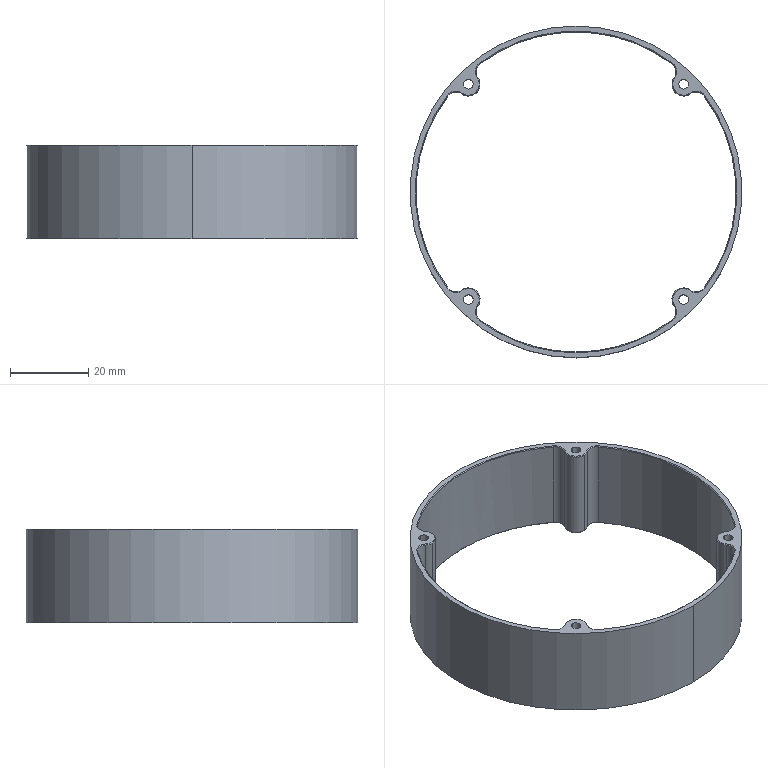NC program | NX | posted with a generic post | part box 85 x 85 x 24 mm
Lines 3651 to 4571 of 6793:
(PLANAR_MILL_COPY , TOOL : D4)
N7270 T11 M6
N7272 G54
N7274 G17 G0 G90 X-22.178 Y-27.673 S7000 M3
N7276 G43 Z30. H11
N7278 Z2.5
N7280 G94 G1 Z-0.5 F1000.
N7282 G3 X-22.64 Y-28.366 R1.
N7284 G2 X-23.519 Y-30.498 R5.
N7286 G3 X-23.413 Y-31.19 R0.5
N7288 X-21.071 Y-32.818 R39.
N7290 X-20.172 Y-32.91 R1.
N7292 G1 Z2.5
N7294 G0 X-22.178 Y-27.673 Z2.
N7296 G1 Z-1.
N7298 G3 X-22.64 Y-28.366 R1.
N7300 G2 X-23.519 Y-30.498 R5.
N7302 G3 X-23.413 Y-31.19 R0.5
N7304 X-21.071 Y-32.818 R39.
N7306 X-20.172 Y-32.91 R1.
N7308 G1 Z2.
N7310 G0 X-22.178 Y-27.673 Z1.5
N7312 G1 Z-1.5
N7314 G3 X-22.64 Y-28.366 R1.
N7316 G2 X-23.519 Y-30.498 R5.
N7318 G3 X-23.413 Y-31.19 R0.5
N7320 X-21.071 Y-32.818 R39.
N7322 X-20.172 Y-32.91 R1.
N7324 G1 Z1.5
N7326 G0 X-22.178 Y-27.673 Z1.
N7328 G1 Z-2.
N7330 G3 X-22.64 Y-28.366 R1.
N7332 G2 X-23.519 Y-30.498 R5.
N7334 G3 X-23.413 Y-31.19 R0.5
N7336 X-21.071 Y-32.818 R39.
N7338 X-20.172 Y-32.91 R1.
N7340 G1 Z1.
N7342 G0 X-22.178 Y-27.673 Z0.5
N7344 G1 Z-2.5
N7346 G3 X-22.64 Y-28.366 R1.
N7348 G2 X-23.519 Y-30.498 R5.
N7350 G3 X-23.413 Y-31.19 R0.5
N7352 X-21.071 Y-32.818 R39.
N7354 X-20.172 Y-32.91 R1.
N7356 G1 Z0.5
N7358 G0 X-22.178 Y-27.673 Z0.
N7360 G1 Z-3.
N7362 G3 X-22.64 Y-28.366 R1.
N7364 G2 X-23.519 Y-30.498 R5.
N7366 G3 X-23.413 Y-31.19 R0.5
N7368 X-21.071 Y-32.818 R39.
N7370 X-20.172 Y-32.91 R1.
N7372 G1 Z0.
N7374 G0 X-22.178 Y-27.673 Z-0.5
N7376 G1 Z-3.5
N7378 G3 X-22.64 Y-28.366 R1.
N7380 G2 X-23.519 Y-30.498 R5.
N7382 G3 X-23.413 Y-31.19 R0.5
N7384 X-21.071 Y-32.818 R39.
N7386 X-20.172 Y-32.91 R1.
N7388 G1 Z-0.5
N7390 G0 X-22.178 Y-27.673 Z-1.
N7392 G1 Z-4.
N7394 G3 X-22.64 Y-28.366 R1.
N7396 G2 X-23.519 Y-30.498 R5.
N7398 G3 X-23.413 Y-31.19 R0.5
N7400 X-21.071 Y-32.818 R39.
N7402 X-20.172 Y-32.91 R1.
N7404 G1 Z-1.
N7406 G0 X-22.178 Y-27.673 Z-1.5
N7408 G1 Z-4.5
N7410 G3 X-22.64 Y-28.366 R1.
N7412 G2 X-23.519 Y-30.498 R5.
N7414 G3 X-23.413 Y-31.19 R0.5
N7416 X-21.071 Y-32.818 R39.
N7418 X-20.172 Y-32.91 R1.
N7420 G1 Z-1.5
N7422 G0 X-22.178 Y-27.673 Z-2.
N7424 G1 Z-5.
N7426 G3 X-22.64 Y-28.366 R1.
N7428 G2 X-23.519 Y-30.498 R5.
N7430 G3 X-23.413 Y-31.19 R0.5
N7432 X-21.071 Y-32.818 R39.
N7434 X-20.172 Y-32.91 R1.
N7436 G1 Z-2.
N7438 G0 X-22.178 Y-27.673 Z-2.5
N7440 G1 Z-5.5
N7442 G3 X-22.64 Y-28.366 R1.
N7444 G2 X-23.519 Y-30.498 R5.
N7446 G3 X-23.413 Y-31.19 R0.5
N7448 X-21.071 Y-32.818 R39.
N7450 X-20.172 Y-32.91 R1.
N7452 G1 Z-2.5
N7454 G0 X-22.178 Y-27.673 Z-3.
N7456 G1 Z-6.
N7458 G3 X-22.64 Y-28.366 R1.
N7460 G2 X-23.519 Y-30.498 R5.
N7462 G3 X-23.413 Y-31.19 R0.5
N7464 X-21.071 Y-32.818 R39.
N7466 X-20.172 Y-32.91 R1.
N7468 G1 Z-3.
N7470 G0 X-22.178 Y-27.673 Z-3.5
N7472 G1 Z-6.5
N7474 G3 X-22.64 Y-28.366 R1.
N7476 G2 X-23.519 Y-30.498 R5.
N7478 G3 X-23.413 Y-31.19 R0.5
N7480 X-21.071 Y-32.818 R39.
N7482 X-20.172 Y-32.91 R1.
N7484 G1 Z-3.5
N7486 G0 X-22.178 Y-27.673 Z-4.
N7488 G1 Z-7.
N7490 G3 X-22.64 Y-28.366 R1.
N7492 G2 X-23.519 Y-30.498 R5.
N7494 G3 X-23.413 Y-31.19 R0.5
N7496 X-21.071 Y-32.818 R39.
N7498 X-20.172 Y-32.91 R1.
N7500 G1 Z-4.
N7502 G0 X-22.178 Y-27.673 Z-4.5
N7504 G1 Z-7.5
N7506 G3 X-22.64 Y-28.366 R1.
N7508 G2 X-23.519 Y-30.498 R5.
N7510 G3 X-23.413 Y-31.19 R0.5
N7512 X-21.071 Y-32.818 R39.
N7514 X-20.172 Y-32.91 R1.
N7516 G1 Z-4.5
N7518 G0 X-22.178 Y-27.673 Z-5.
N7520 G1 Z-8.
N7522 G3 X-22.64 Y-28.366 R1.
N7524 G2 X-23.519 Y-30.498 R5.
N7526 G3 X-23.413 Y-31.19 R0.5
N7528 X-21.071 Y-32.818 R39.
N7530 X-20.172 Y-32.91 R1.
N7532 G1 Z-5.
N7534 G0 X-22.178 Y-27.673 Z-5.5
N7536 G1 Z-8.5
N7538 G3 X-22.64 Y-28.366 R1.
N7540 G2 X-23.519 Y-30.498 R5.
N7542 G3 X-23.413 Y-31.19 R0.5
N7544 X-21.071 Y-32.818 R39.
N7546 X-20.172 Y-32.91 R1.
N7548 G1 Z-5.5
N7550 G0 X-22.178 Y-27.673 Z-6.
N7552 G1 Z-9.
N7554 G3 X-22.64 Y-28.366 R1.
N7556 G2 X-23.519 Y-30.498 R5.
N7558 G3 X-23.413 Y-31.19 R0.5
N7560 X-21.071 Y-32.818 R39.
N7562 X-20.172 Y-32.91 R1.
N7564 G1 Z-6.
N7566 G0 X-22.178 Y-27.673 Z-6.5
N7568 G1 Z-9.5
N7570 G3 X-22.64 Y-28.366 R1.
N7572 G2 X-23.519 Y-30.498 R5.
N7574 G3 X-23.413 Y-31.19 R0.5
N7576 X-21.071 Y-32.818 R39.
N7578 X-20.172 Y-32.91 R1.
N7580 G1 Z-6.5
N7582 G0 X-22.178 Y-27.673 Z-7.
N7584 G1 Z-10.
N7586 G3 X-22.64 Y-28.366 R1.
N7588 G2 X-23.519 Y-30.498 R5.
N7590 G3 X-23.413 Y-31.19 R0.5
N7592 X-21.071 Y-32.818 R39.
N7594 X-20.172 Y-32.91 R1.
N7596 G1 Z-7.
N7598 G0 X-22.178 Y-27.673 Z-7.5
N7600 G1 Z-10.5
N7602 G3 X-22.64 Y-28.366 R1.
N7604 G2 X-23.519 Y-30.498 R5.
N7606 G3 X-23.413 Y-31.19 R0.5
N7608 X-21.071 Y-32.818 R39.
N7610 X-20.172 Y-32.91 R1.
N7612 G1 Z-7.5
N7614 G0 X-22.178 Y-27.673 Z-8.
N7616 G1 Z-11.
N7618 G3 X-22.64 Y-28.366 R1.
N7620 G2 X-23.519 Y-30.498 R5.
N7622 G3 X-23.413 Y-31.19 R0.5
N7624 X-21.071 Y-32.818 R39.
N7626 X-20.172 Y-32.91 R1.
N7628 G1 Z-8.
N7630 G0 X-22.178 Y-27.673 Z-8.5
N7632 G1 Z-11.5
N7634 G3 X-22.64 Y-28.366 R1.
N7636 G2 X-23.519 Y-30.498 R5.
N7638 G3 X-23.413 Y-31.19 R0.5
N7640 X-21.071 Y-32.818 R39.
N7642 X-20.172 Y-32.91 R1.
N7644 G1 Z-8.5
N7646 G0 X-22.178 Y-27.673 Z-9.
N7648 G1 Z-12.
N7650 G3 X-22.64 Y-28.366 R1.
N7652 G2 X-23.519 Y-30.498 R5.
N7654 G3 X-23.413 Y-31.19 R0.5
N7656 X-21.071 Y-32.818 R39.
N7658 X-20.172 Y-32.91 R1.
N7660 G1 Z-9.
N7662 G0 X-22.178 Y-27.673 Z-9.5
N7664 G1 Z-12.5
N7666 G3 X-22.64 Y-28.366 R1.
N7668 G2 X-23.519 Y-30.498 R5.
N7670 G3 X-23.413 Y-31.19 R0.5
N7672 X-21.071 Y-32.818 R39.
N7674 X-20.172 Y-32.91 R1.
N7676 G1 Z-9.5
N7678 G0 X-22.178 Y-27.673 Z-10.
N7680 G1 Z-13.
N7682 G3 X-22.64 Y-28.366 R1.
N7684 G2 X-23.519 Y-30.498 R5.
N7686 G3 X-23.413 Y-31.19 R0.5
N7688 X-21.071 Y-32.818 R39.
N7690 X-20.172 Y-32.91 R1.
N7692 G1 Z-10.
N7694 G0 X-22.178 Y-27.673 Z-10.5
N7696 G1 Z-13.5
N7698 G3 X-22.64 Y-28.366 R1.
N7700 G2 X-23.519 Y-30.498 R5.
N7702 G3 X-23.413 Y-31.19 R0.5
N7704 X-21.071 Y-32.818 R39.
N7706 X-20.172 Y-32.91 R1.
N7708 G1 Z-10.5
N7710 G0 X-22.178 Y-27.673 Z-11.
N7712 G1 Z-14.
N7714 G3 X-22.64 Y-28.366 R1.
N7716 G2 X-23.519 Y-30.498 R5.
N7718 G3 X-23.413 Y-31.19 R0.5
N7720 X-21.071 Y-32.818 R39.
N7722 X-20.172 Y-32.91 R1.
N7724 G1 Z-11.
N7726 G0 X-22.178 Y-27.673 Z-11.5
N7728 G1 Z-14.5
N7730 G3 X-22.64 Y-28.366 R1.
N7732 G2 X-23.519 Y-30.498 R5.
N7734 G3 X-23.413 Y-31.19 R0.5
N7736 X-21.071 Y-32.818 R39.
N7738 X-20.172 Y-32.91 R1.
N7740 G1 Z-11.5
N7742 G0 X-22.178 Y-27.673 Z-12.
N7744 G1 Z-15.
N7746 G3 X-22.64 Y-28.366 R1.
N7748 G2 X-23.519 Y-30.498 R5.
N7750 G3 X-23.413 Y-31.19 R0.5
N7752 X-21.071 Y-32.818 R39.
N7754 X-20.172 Y-32.91 R1.
N7756 G1 Z-12.
N7758 G0 X-22.178 Y-27.673 Z-12.5
N7760 G1 Z-15.5
N7762 G3 X-22.64 Y-28.366 R1.
N7764 G2 X-23.519 Y-30.498 R5.
N7766 G3 X-23.413 Y-31.19 R0.5
N7768 X-21.071 Y-32.818 R39.
N7770 X-20.172 Y-32.91 R1.
N7772 G1 Z-12.5
N7774 G0 X-22.178 Y-27.673 Z-13.
N7776 G1 Z-16.
N7778 G3 X-22.64 Y-28.366 R1.
N7780 G2 X-23.519 Y-30.498 R5.
N7782 G3 X-23.413 Y-31.19 R0.5
N7784 X-21.071 Y-32.818 R39.
N7786 X-20.172 Y-32.91 R1.
N7788 G1 Z-13.
N7790 G0 X-22.178 Y-27.673 Z-13.5
N7792 G1 Z-16.5
N7794 G3 X-22.64 Y-28.366 R1.
N7796 G2 X-23.519 Y-30.498 R5.
N7798 G3 X-23.413 Y-31.19 R0.5
N7800 X-21.071 Y-32.818 R39.
N7802 X-20.172 Y-32.91 R1.
N7804 G1 Z-13.5
N7806 G0 X-22.178 Y-27.673 Z-14.
N7808 G1 Z-17.
N7810 G3 X-22.64 Y-28.366 R1.
N7812 G2 X-23.519 Y-30.498 R5.
N7814 G3 X-23.413 Y-31.19 R0.5
N7816 X-21.071 Y-32.818 R39.
N7818 X-20.172 Y-32.91 R1.
N7820 G1 Z-14.
N7822 G0 X-22.178 Y-27.673 Z-14.5
N7824 G1 Z-17.5
N7826 G3 X-22.64 Y-28.366 R1.
N7828 G2 X-23.519 Y-30.498 R5.
N7830 G3 X-23.413 Y-31.19 R0.5
N7832 X-21.071 Y-32.818 R39.
N7834 X-20.172 Y-32.91 R1.
N7836 G1 Z-14.5
N7838 G0 X-22.178 Y-27.673 Z-15.
N7840 G1 Z-18.
N7842 G3 X-22.64 Y-28.366 R1.
N7844 G2 X-23.519 Y-30.498 R5.
N7846 G3 X-23.413 Y-31.19 R0.5
N7848 X-21.071 Y-32.818 R39.
N7850 X-20.172 Y-32.91 R1.
N7852 G1 Z-15.
N7854 G0 X-22.178 Y-27.673 Z-15.5
N7856 G1 Z-18.5
N7858 G3 X-22.64 Y-28.366 R1.
N7860 G2 X-23.519 Y-30.498 R5.
N7862 G3 X-23.413 Y-31.19 R0.5
N7864 X-21.071 Y-32.818 R39.
N7866 X-20.172 Y-32.91 R1.
N7868 G1 Z-15.5
N7870 G0 X-22.178 Y-27.673 Z-16.
N7872 G1 Z-19.
N7874 G3 X-22.64 Y-28.366 R1.
N7876 G2 X-23.519 Y-30.498 R5.
N7878 G3 X-23.413 Y-31.19 R0.5
N7880 X-21.071 Y-32.818 R39.
N7882 X-20.172 Y-32.91 R1.
N7884 G1 Z-16.
N7886 G0 X-22.178 Y-27.673 Z-16.5
N7888 G1 Z-19.5
N7890 G3 X-22.64 Y-28.366 R1.
N7892 G2 X-23.519 Y-30.498 R5.
N7894 G3 X-23.413 Y-31.19 R0.5
N7896 X-21.071 Y-32.818 R39.
N7898 X-20.172 Y-32.91 R1.
N7900 G1 Z-16.5
N7902 G0 X-22.178 Y-27.673 Z-17.
N7904 G1 Z-20.
N7906 G3 X-22.64 Y-28.366 R1.
N7908 G2 X-23.519 Y-30.498 R5.
N7910 G3 X-23.413 Y-31.19 R0.5
N7912 X-21.071 Y-32.818 R39.
N7914 X-20.172 Y-32.91 R1.
N7916 G1 Z-17.
N7918 G0 X-22.178 Y-27.673 Z-17.5
N7920 G1 Z-20.5
N7922 G3 X-22.64 Y-28.366 R1.
N7924 G2 X-23.519 Y-30.498 R5.
N7926 G3 X-23.413 Y-31.19 R0.5
N7928 X-21.071 Y-32.818 R39.
N7930 X-20.172 Y-32.91 R1.
N7932 G1 Z-17.5
N7934 G0 X-22.178 Y-27.673 Z-18.
N7936 G1 Z-21.
N7938 G3 X-22.64 Y-28.366 R1.
N7940 G2 X-23.519 Y-30.498 R5.
N7942 G3 X-23.413 Y-31.19 R0.5
N7944 X-21.071 Y-32.818 R39.
N7946 X-20.172 Y-32.91 R1.
N7948 G1 Z-18.
N7950 G0 X-22.178 Y-27.673 Z-18.5
N7952 G1 Z-21.5
N7954 G3 X-22.64 Y-28.366 R1.
N7956 G2 X-23.519 Y-30.498 R5.
N7958 G3 X-23.413 Y-31.19 R0.5
N7960 X-21.071 Y-32.818 R39.
N7962 X-20.172 Y-32.91 R1.
N7964 G1 Z-18.5
N7966 G0 X-22.178 Y-27.673 Z-19.
N7968 G1 Z-22.
N7970 G3 X-22.64 Y-28.366 R1.
N7972 G2 X-23.519 Y-30.498 R5.
N7974 G3 X-23.413 Y-31.19 R0.5
N7976 X-21.071 Y-32.818 R39.
N7978 X-20.172 Y-32.91 R1.
N7980 G1 Z-19.
N7982 G0 X-22.178 Y-27.673 Z-19.5
N7984 G1 Z-22.5
N7986 G3 X-22.64 Y-28.366 R1.
N7988 G2 X-23.519 Y-30.498 R5.
N7990 G3 X-23.413 Y-31.19 R0.5
N7992 X-21.071 Y-32.818 R39.
N7994 X-20.172 Y-32.91 R1.
N7996 G1 Z-19.5
N7998 G0 X-22.178 Y-27.673 Z-20.
N8000 G1 Z-23.
N8002 G3 X-22.64 Y-28.366 R1.
N8004 G2 X-23.519 Y-30.498 R5.
N8006 G3 X-23.413 Y-31.19 R0.5
N8008 X-21.071 Y-32.818 R39.
N8010 X-20.172 Y-32.91 R1.
N8012 G1 Z-20.
N8014 G0 X-22.178 Y-27.673 Z-20.5
N8016 G1 Z-23.5
N8018 G3 X-22.64 Y-28.366 R1.
N8020 G2 X-23.519 Y-30.498 R5.
N8022 G3 X-23.413 Y-31.19 R0.5
N8024 X-21.071 Y-32.818 R39.
N8026 X-20.172 Y-32.91 R1.
N8028 G1 Z-20.5
N8030 G0 X-22.178 Y-27.673 Z-21.
N8032 G1 Z-24.
N8034 G3 X-22.64 Y-28.366 R1.
N8036 G2 X-23.519 Y-30.498 R5.
N8038 G3 X-23.413 Y-31.19 R0.5
N8040 X-21.071 Y-32.818 R39.
N8042 X-20.172 Y-32.91 R1.
N8044 G1 Z-21.
N8046 G0 Z30.
N8048 X-32.91 Y-20.172
N8050 Z2.5
N8052 G1 Z-0.5
N8054 G3 X-32.818 Y-21.071 R1.
N8056 X-31.19 Y-23.413 R39.
N8058 X-30.498 Y-23.519 R0.5
N8060 G2 X-28.366 Y-22.64 R5.
N8062 G3 X-27.673 Y-22.178 R1.
N8064 G1 Z2.5
N8066 G0 X-32.91 Y-20.172 Z2.
N8068 G1 Z-1.
N8070 G3 X-32.818 Y-21.071 R1.
N8072 X-31.19 Y-23.413 R39.
N8074 X-30.498 Y-23.519 R0.5
N8076 G2 X-28.366 Y-22.64 R5.
N8078 G3 X-27.673 Y-22.178 R1.
N8080 G1 Z2.
N8082 G0 X-32.91 Y-20.172 Z1.5
N8084 G1 Z-1.5
N8086 G3 X-32.818 Y-21.071 R1.
N8088 X-31.19 Y-23.413 R39.
N8090 X-30.498 Y-23.519 R0.5
N8092 G2 X-28.366 Y-22.64 R5.
N8094 G3 X-27.673 Y-22.178 R1.
N8096 G1 Z1.5
N8098 G0 X-32.91 Y-20.172 Z1.
N8100 G1 Z-2.
N8102 G3 X-32.818 Y-21.071 R1.
N8104 X-31.19 Y-23.413 R39.
N8106 X-30.498 Y-23.519 R0.5
N8108 G2 X-28.366 Y-22.64 R5.
N8110 G3 X-27.673 Y-22.178 R1.
N8112 G1 Z1.
N8114 G0 X-32.91 Y-20.172 Z0.5
N8116 G1 Z-2.5
N8118 G3 X-32.818 Y-21.071 R1.
N8120 X-31.19 Y-23.413 R39.
N8122 X-30.498 Y-23.519 R0.5
N8124 G2 X-28.366 Y-22.64 R5.
N8126 G3 X-27.673 Y-22.178 R1.
N8128 G1 Z0.5
N8130 G0 X-32.91 Y-20.172 Z0.
N8132 G1 Z-3.
N8134 G3 X-32.818 Y-21.071 R1.
N8136 X-31.19 Y-23.413 R39.
N8138 X-30.498 Y-23.519 R0.5
N8140 G2 X-28.366 Y-22.64 R5.
N8142 G3 X-27.673 Y-22.178 R1.
N8144 G1 Z0.
N8146 G0 X-32.91 Y-20.172 Z-0.5
N8148 G1 Z-3.5
N8150 G3 X-32.818 Y-21.071 R1.
N8152 X-31.19 Y-23.413 R39.
N8154 X-30.498 Y-23.519 R0.5
N8156 G2 X-28.366 Y-22.64 R5.
N8158 G3 X-27.673 Y-22.178 R1.
N8160 G1 Z-0.5
N8162 G0 X-32.91 Y-20.172 Z-1.
N8164 G1 Z-4.
N8166 G3 X-32.818 Y-21.071 R1.
N8168 X-31.19 Y-23.413 R39.
N8170 X-30.498 Y-23.519 R0.5
N8172 G2 X-28.366 Y-22.64 R5.
N8174 G3 X-27.673 Y-22.178 R1.
N8176 G1 Z-1.
N8178 G0 X-32.91 Y-20.172 Z-1.5
N8180 G1 Z-4.5
N8182 G3 X-32.818 Y-21.071 R1.
N8184 X-31.19 Y-23.413 R39.
N8186 X-30.498 Y-23.519 R0.5
N8188 G2 X-28.366 Y-22.64 R5.
N8190 G3 X-27.673 Y-22.178 R1.
N8192 G1 Z-1.5
N8194 G0 X-32.91 Y-20.172 Z-2.
N8196 G1 Z-5.
N8198 G3 X-32.818 Y-21.071 R1.
N8200 X-31.19 Y-23.413 R39.
N8202 X-30.498 Y-23.519 R0.5
N8204 G2 X-28.366 Y-22.64 R5.
N8206 G3 X-27.673 Y-22.178 R1.
N8208 G1 Z-2.
N8210 G0 X-32.91 Y-20.172 Z-2.5
N8212 G1 Z-5.5
N8214 G3 X-32.818 Y-21.071 R1.
N8216 X-31.19 Y-23.413 R39.
N8218 X-30.498 Y-23.519 R0.5
N8220 G2 X-28.366 Y-22.64 R5.
N8222 G3 X-27.673 Y-22.178 R1.
N8224 G1 Z-2.5
N8226 G0 X-32.91 Y-20.172 Z-3.
N8228 G1 Z-6.
N8230 G3 X-32.818 Y-21.071 R1.
N8232 X-31.19 Y-23.413 R39.
N8234 X-30.498 Y-23.519 R0.5
N8236 G2 X-28.366 Y-22.64 R5.
N8238 G3 X-27.673 Y-22.178 R1.
N8240 G1 Z-3.
N8242 G0 X-32.91 Y-20.172 Z-3.5
N8244 G1 Z-6.5
N8246 G3 X-32.818 Y-21.071 R1.
N8248 X-31.19 Y-23.413 R39.
N8250 X-30.498 Y-23.519 R0.5
N8252 G2 X-28.366 Y-22.64 R5.
N8254 G3 X-27.673 Y-22.178 R1.
N8256 G1 Z-3.5
N8258 G0 X-32.91 Y-20.172 Z-4.
N8260 G1 Z-7.
N8262 G3 X-32.818 Y-21.071 R1.
N8264 X-31.19 Y-23.413 R39.
N8266 X-30.498 Y-23.519 R0.5
N8268 G2 X-28.366 Y-22.64 R5.
N8270 G3 X-27.673 Y-22.178 R1.
N8272 G1 Z-4.
N8274 G0 X-32.91 Y-20.172 Z-4.5
N8276 G1 Z-7.5
N8278 G3 X-32.818 Y-21.071 R1.
N8280 X-31.19 Y-23.413 R39.
N8282 X-30.498 Y-23.519 R0.5
N8284 G2 X-28.366 Y-22.64 R5.
N8286 G3 X-27.673 Y-22.178 R1.
N8288 G1 Z-4.5
N8290 G0 X-32.91 Y-20.172 Z-5.
N8292 G1 Z-8.
N8294 G3 X-32.818 Y-21.071 R1.
N8296 X-31.19 Y-23.413 R39.
N8298 X-30.498 Y-23.519 R0.5
N8300 G2 X-28.366 Y-22.64 R5.
N8302 G3 X-27.673 Y-22.178 R1.
N8304 G1 Z-5.
N8306 G0 X-32.91 Y-20.172 Z-5.5
N8308 G1 Z-8.5
N8310 G3 X-32.818 Y-21.071 R1.
N8312 X-31.19 Y-23.413 R39.
N8314 X-30.498 Y-23.519 R0.5
N8316 G2 X-28.366 Y-22.64 R5.
N8318 G3 X-27.673 Y-22.178 R1.
N8320 G1 Z-5.5
N8322 G0 X-32.91 Y-20.172 Z-6.
N8324 G1 Z-9.
N8326 G3 X-32.818 Y-21.071 R1.
N8328 X-31.19 Y-23.413 R39.
N8330 X-30.498 Y-23.519 R0.5
N8332 G2 X-28.366 Y-22.64 R5.
N8334 G3 X-27.673 Y-22.178 R1.
N8336 G1 Z-6.
N8338 G0 X-32.91 Y-20.172 Z-6.5
N8340 G1 Z-9.5
N8342 G3 X-32.818 Y-21.071 R1.
N8344 X-31.19 Y-23.413 R39.
N8346 X-30.498 Y-23.519 R0.5
N8348 G2 X-28.366 Y-22.64 R5.
N8350 G3 X-27.673 Y-22.178 R1.
N8352 G1 Z-6.5
N8354 G0 X-32.91 Y-20.172 Z-7.
N8356 G1 Z-10.
N8358 G3 X-32.818 Y-21.071 R1.
N8360 X-31.19 Y-23.413 R39.
N8362 X-30.498 Y-23.519 R0.5
N8364 G2 X-28.366 Y-22.64 R5.
N8366 G3 X-27.673 Y-22.178 R1.
N8368 G1 Z-7.
N8370 G0 X-32.91 Y-20.172 Z-7.5
N8372 G1 Z-10.5
N8374 G3 X-32.818 Y-21.071 R1.
N8376 X-31.19 Y-23.413 R39.
N8378 X-30.498 Y-23.519 R0.5
N8380 G2 X-28.366 Y-22.64 R5.
N8382 G3 X-27.673 Y-22.178 R1.
N8384 G1 Z-7.5
N8386 G0 X-32.91 Y-20.172 Z-8.
N8388 G1 Z-11.
N8390 G3 X-32.818 Y-21.071 R1.
N8392 X-31.19 Y-23.413 R39.
N8394 X-30.498 Y-23.519 R0.5
N8396 G2 X-28.366 Y-22.64 R5.
N8398 G3 X-27.673 Y-22.178 R1.
N8400 G1 Z-8.
N8402 G0 X-32.91 Y-20.172 Z-8.5
N8404 G1 Z-11.5
N8406 G3 X-32.818 Y-21.071 R1.
N8408 X-31.19 Y-23.413 R39.
N8410 X-30.498 Y-23.519 R0.5
N8412 G2 X-28.366 Y-22.64 R5.
N8414 G3 X-27.673 Y-22.178 R1.
N8416 G1 Z-8.5
N8418 G0 X-32.91 Y-20.172 Z-9.
N8420 G1 Z-12.
N8422 G3 X-32.818 Y-21.071 R1.
N8424 X-31.19 Y-23.413 R39.
N8426 X-30.498 Y-23.519 R0.5
N8428 G2 X-28.366 Y-22.64 R5.
N8430 G3 X-27.673 Y-22.178 R1.
N8432 G1 Z-9.
N8434 G0 X-32.91 Y-20.172 Z-9.5
N8436 G1 Z-12.5
N8438 G3 X-32.818 Y-21.071 R1.
N8440 X-31.19 Y-23.413 R39.
N8442 X-30.498 Y-23.519 R0.5
N8444 G2 X-28.366 Y-22.64 R5.
N8446 G3 X-27.673 Y-22.178 R1.
N8448 G1 Z-9.5
N8450 G0 X-32.91 Y-20.172 Z-10.
N8452 G1 Z-13.
N8454 G3 X-32.818 Y-21.071 R1.
N8456 X-31.19 Y-23.413 R39.
N8458 X-30.498 Y-23.519 R0.5
N8460 G2 X-28.366 Y-22.64 R5.
N8462 G3 X-27.673 Y-22.178 R1.
N8464 G1 Z-10.
N8466 G0 X-32.91 Y-20.172 Z-10.5
N8468 G1 Z-13.5
N8470 G3 X-32.818 Y-21.071 R1.
N8472 X-31.19 Y-23.413 R39.
N8474 X-30.498 Y-23.519 R0.5
N8476 G2 X-28.366 Y-22.64 R5.
N8478 G3 X-27.673 Y-22.178 R1.
N8480 G1 Z-10.5
N8482 G0 X-32.91 Y-20.172 Z-11.
N8484 G1 Z-14.
N8486 G3 X-32.818 Y-21.071 R1.
N8488 X-31.19 Y-23.413 R39.
N8490 X-30.498 Y-23.519 R0.5
N8492 G2 X-28.366 Y-22.64 R5.
N8494 G3 X-27.673 Y-22.178 R1.
N8496 G1 Z-11.
N8498 G0 X-32.91 Y-20.172 Z-11.5
N8500 G1 Z-14.5
N8502 G3 X-32.818 Y-21.071 R1.
N8504 X-31.19 Y-23.413 R39.
N8506 X-30.498 Y-23.519 R0.5
N8508 G2 X-28.366 Y-22.64 R5.
N8510 G3 X-27.673 Y-22.178 R1.
N8512 G1 Z-11.5
N8514 G0 X-32.91 Y-20.172 Z-12.
N8516 G1 Z-15.
N8518 G3 X-32.818 Y-21.071 R1.
N8520 X-31.19 Y-23.413 R39.
N8522 X-30.498 Y-23.519 R0.5
N8524 G2 X-28.366 Y-22.64 R5.
N8526 G3 X-27.673 Y-22.178 R1.
N8528 G1 Z-12.
N8530 G0 X-32.91 Y-20.172 Z-12.5
N8532 G1 Z-15.5
N8534 G3 X-32.818 Y-21.071 R1.
N8536 X-31.19 Y-23.413 R39.
N8538 X-30.498 Y-23.519 R0.5
N8540 G2 X-28.366 Y-22.64 R5.
N8542 G3 X-27.673 Y-22.178 R1.
N8544 G1 Z-12.5
N8546 G0 X-32.91 Y-20.172 Z-13.
N8548 G1 Z-16.
N8550 G3 X-32.818 Y-21.071 R1.
N8552 X-31.19 Y-23.413 R39.
N8554 X-30.498 Y-23.519 R0.5
N8556 G2 X-28.366 Y-22.64 R5.
N8558 G3 X-27.673 Y-22.178 R1.
N8560 G1 Z-13.
N8562 G0 X-32.91 Y-20.172 Z-13.5
N8564 G1 Z-16.5
N8566 G3 X-32.818 Y-21.071 R1.
N8568 X-31.19 Y-23.413 R39.
N8570 X-30.498 Y-23.519 R0.5
N8572 G2 X-28.366 Y-22.64 R5.
N8574 G3 X-27.673 Y-22.178 R1.
N8576 G1 Z-13.5
N8578 G0 X-32.91 Y-20.172 Z-14.
N8580 G1 Z-17.
N8582 G3 X-32.818 Y-21.071 R1.
N8584 X-31.19 Y-23.413 R39.
N8586 X-30.498 Y-23.519 R0.5
N8588 G2 X-28.366 Y-22.64 R5.
N8590 G3 X-27.673 Y-22.178 R1.
N8592 G1 Z-14.
N8594 G0 X-32.91 Y-20.172 Z-14.5
N8596 G1 Z-17.5
N8598 G3 X-32.818 Y-21.071 R1.
N8600 X-31.19 Y-23.413 R39.
N8602 X-30.498 Y-23.519 R0.5
N8604 G2 X-28.366 Y-22.64 R5.
N8606 G3 X-27.673 Y-22.178 R1.
N8608 G1 Z-14.5
N8610 G0 X-32.91 Y-20.172 Z-15.
N8612 G1 Z-18.
N8614 G3 X-32.818 Y-21.071 R1.
N8616 X-31.19 Y-23.413 R39.
N8618 X-30.498 Y-23.519 R0.5
N8620 G2 X-28.366 Y-22.64 R5.
N8622 G3 X-27.673 Y-22.178 R1.
N8624 G1 Z-15.
N8626 G0 X-32.91 Y-20.172 Z-15.5
N8628 G1 Z-18.5
N8630 G3 X-32.818 Y-21.071 R1.
N8632 X-31.19 Y-23.413 R39.
N8634 X-30.498 Y-23.519 R0.5
N8636 G2 X-28.366 Y-22.64 R5.
N8638 G3 X-27.673 Y-22.178 R1.
N8640 G1 Z-15.5
N8642 G0 X-32.91 Y-20.172 Z-16.
N8644 G1 Z-19.
N8646 G3 X-32.818 Y-21.071 R1.
N8648 X-31.19 Y-23.413 R39.
N8650 X-30.498 Y-23.519 R0.5
N8652 G2 X-28.366 Y-22.64 R5.
N8654 G3 X-27.673 Y-22.178 R1.
N8656 G1 Z-16.
N8658 G0 X-32.91 Y-20.172 Z-16.5
N8660 G1 Z-19.5
N8662 G3 X-32.818 Y-21.071 R1.
N8664 X-31.19 Y-23.413 R39.
N8666 X-30.498 Y-23.519 R0.5
N8668 G2 X-28.366 Y-22.64 R5.
N8670 G3 X-27.673 Y-22.178 R1.
N8672 G1 Z-16.5
N8674 G0 X-32.91 Y-20.172 Z-17.
N8676 G1 Z-20.
N8678 G3 X-32.818 Y-21.071 R1.
N8680 X-31.19 Y-23.413 R39.
N8682 X-30.498 Y-23.519 R0.5
N8684 G2 X-28.366 Y-22.64 R5.
N8686 G3 X-27.673 Y-22.178 R1.
N8688 G1 Z-17.
N8690 G0 X-32.91 Y-20.172 Z-17.5
N8692 G1 Z-20.5
N8694 G3 X-32.818 Y-21.071 R1.
N8696 X-31.19 Y-23.413 R39.
N8698 X-30.498 Y-23.519 R0.5
N8700 G2 X-28.366 Y-22.64 R5.
N8702 G3 X-27.673 Y-22.178 R1.
N8704 G1 Z-17.5
N8706 G0 X-32.91 Y-20.172 Z-18.
N8708 G1 Z-21.
N8710 G3 X-32.818 Y-21.071 R1.
N8712 X-31.19 Y-23.413 R39.
N8714 X-30.498 Y-23.519 R0.5
N8716 G2 X-28.366 Y-22.64 R5.
N8718 G3 X-27.673 Y-22.178 R1.
N8720 G1 Z-18.
N8722 G0 X-32.91 Y-20.172 Z-18.5
N8724 G1 Z-21.5
N8726 G3 X-32.818 Y-21.071 R1.
N8728 X-31.19 Y-23.413 R39.
N8730 X-30.498 Y-23.519 R0.5
N8732 G2 X-28.366 Y-22.64 R5.
N8734 G3 X-27.673 Y-22.178 R1.
N8736 G1 Z-18.5
N8738 G0 X-32.91 Y-20.172 Z-19.
N8740 G1 Z-22.
N8742 G3 X-32.818 Y-21.071 R1.
N8744 X-31.19 Y-23.413 R39.
N8746 X-30.498 Y-23.519 R0.5
N8748 G2 X-28.366 Y-22.64 R5.
N8750 G3 X-27.673 Y-22.178 R1.
N8752 G1 Z-19.
N8754 G0 X-32.91 Y-20.172 Z-19.5
N8756 G1 Z-22.5
N8758 G3 X-32.818 Y-21.071 R1.
N8760 X-31.19 Y-23.413 R39.
N8762 X-30.498 Y-23.519 R0.5
N8764 G2 X-28.366 Y-22.64 R5.
N8766 G3 X-27.673 Y-22.178 R1.
N8768 G1 Z-19.5
N8770 G0 X-32.91 Y-20.172 Z-20.
N8772 G1 Z-23.
N8774 G3 X-32.818 Y-21.071 R1.
N8776 X-31.19 Y-23.413 R39.
N8778 X-30.498 Y-23.519 R0.5
N8780 G2 X-28.366 Y-22.64 R5.
N8782 G3 X-27.673 Y-22.178 R1.
N8784 G1 Z-20.
N8786 G0 X-32.91 Y-20.172 Z-20.5
N8788 G1 Z-23.5
N8790 G3 X-32.818 Y-21.071 R1.
N8792 X-31.19 Y-23.413 R39.
N8794 X-30.498 Y-23.519 R0.5
N8796 G2 X-28.366 Y-22.64 R5.
N8798 G3 X-27.673 Y-22.178 R1.
N8800 G1 Z-20.5
N8802 G0 X-32.91 Y-20.172 Z-21.
N8804 G1 Z-24.
N8806 G3 X-32.818 Y-21.071 R1.
N8808 X-31.19 Y-23.413 R39.
N8810 X-30.498 Y-23.519 R0.5
N8812 G2 X-28.366 Y-22.64 R5.
N8814 G3 X-27.673 Y-22.178 R1.
N8816 G1 Z-21.
N8818 G0 Z30.
N8820 Y22.178
N8822 Z2.5
N8824 G1 Z-0.5
N8826 G3 X-28.366 Y22.64 R1.
N8828 G2 X-30.498 Y23.519 R5.
N8830 G3 X-31.19 Y23.413 R0.5
N8832 X-32.818 Y21.071 R39.
N8834 X-32.91 Y20.172 R1.
N8836 G1 Z2.5
N8838 G0 X-27.673 Y22.178 Z2.
N8840 G1 Z-1.
N8842 G3 X-28.366 Y22.64 R1.
N8844 G2 X-30.498 Y23.519 R5.
N8846 G3 X-31.19 Y23.413 R0.5
N8848 X-32.818 Y21.071 R39.
N8850 X-32.91 Y20.172 R1.
N8852 G1 Z2.
N8854 G0 X-27.673 Y22.178 Z1.5
N8856 G1 Z-1.5
N8858 G3 X-28.366 Y22.64 R1.
N8860 G2 X-30.498 Y23.519 R5.
N8862 G3 X-31.19 Y23.413 R0.5
N8864 X-32.818 Y21.071 R39.
N8866 X-32.91 Y20.172 R1.
N8868 G1 Z1.5
N8870 G0 X-27.673 Y22.178 Z1.
N8872 G1 Z-2.
N8874 G3 X-28.366 Y22.64 R1.
N8876 G2 X-30.498 Y23.519 R5.
N8878 G3 X-31.19 Y23.413 R0.5
N8880 X-32.818 Y21.071 R39.
N8882 X-32.91 Y20.172 R1.
N8884 G1 Z1.
N8886 G0 X-27.673 Y22.178 Z0.5
N8888 G1 Z-2.5
N8890 G3 X-28.366 Y22.64 R1.
N8892 G2 X-30.498 Y23.519 R5.
N8894 G3 X-31.19 Y23.413 R0.5
N8896 X-32.818 Y21.071 R39.
N8898 X-32.91 Y20.172 R1.
N8900 G1 Z0.5
N8902 G0 X-27.673 Y22.178 Z0.
N8904 G1 Z-3.
N8906 G3 X-28.366 Y22.64 R1.
N8908 G2 X-30.498 Y23.519 R5.
N8910 G3 X-31.19 Y23.413 R0.5
N8912 X-32.818 Y21.071 R39.
N8914 X-32.91 Y20.172 R1.
N8916 G1 Z0.
N8918 G0 X-27.673 Y22.178 Z-0.5
N8920 G1 Z-3.5
N8922 G3 X-28.366 Y22.64 R1.
N8924 G2 X-30.498 Y23.519 R5.
N8926 G3 X-31.19 Y23.413 R0.5
N8928 X-32.818 Y21.071 R39.
N8930 X-32.91 Y20.172 R1.
N8932 G1 Z-0.5
N8934 G0 X-27.673 Y22.178 Z-1.
N8936 G1 Z-4.
N8938 G3 X-28.366 Y22.64 R1.
N8940 G2 X-30.498 Y23.519 R5.
N8942 G3 X-31.19 Y23.413 R0.5
N8944 X-32.818 Y21.071 R39.
N8946 X-32.91 Y20.172 R1.
N8948 G1 Z-1.
N8950 G0 X-27.673 Y22.178 Z-1.5
N8952 G1 Z-4.5
N8954 G3 X-28.366 Y22.64 R1.
N8956 G2 X-30.498 Y23.519 R5.
N8958 G3 X-31.19 Y23.413 R0.5
N8960 X-32.818 Y21.071 R39.
N8962 X-32.91 Y20.172 R1.
N8964 G1 Z-1.5
N8966 G0 X-27.673 Y22.178 Z-2.
N8968 G1 Z-5.
N8970 G3 X-28.366 Y22.64 R1.
N8972 G2 X-30.498 Y23.519 R5.
N8974 G3 X-31.19 Y23.413 R0.5
N8976 X-32.818 Y21.071 R39.
N8978 X-32.91 Y20.172 R1.
N8980 G1 Z-2.
N8982 G0 X-27.673 Y22.178 Z-2.5
N8984 G1 Z-5.5
N8986 G3 X-28.366 Y22.64 R1.
N8988 G2 X-30.498 Y23.519 R5.
N8990 G3 X-31.19 Y23.413 R0.5
N8992 X-32.818 Y21.071 R39.
N8994 X-32.91 Y20.172 R1.
N8996 G1 Z-2.5
N8998 G0 X-27.673 Y22.178 Z-3.
N9000 G1 Z-6.
N9002 G3 X-28.366 Y22.64 R1.
N9004 G2 X-30.498 Y23.519 R5.
N9006 G3 X-31.19 Y23.413 R0.5
N9008 X-32.818 Y21.071 R39.
N9010 X-32.91 Y20.172 R1.
N9012 G1 Z-3.
N9014 G0 X-27.673 Y22.178 Z-3.5
N9016 G1 Z-6.5
N9018 G3 X-28.366 Y22.64 R1.
N9020 G2 X-30.498 Y23.519 R5.
N9022 G3 X-31.19 Y23.413 R0.5
N9024 X-32.818 Y21.071 R39.
N9026 X-32.91 Y20.172 R1.
N9028 G1 Z-3.5
N9030 G0 X-27.673 Y22.178 Z-4.
N9032 G1 Z-7.
N9034 G3 X-28.366 Y22.64 R1.
N9036 G2 X-30.498 Y23.519 R5.
N9038 G3 X-31.19 Y23.413 R0.5
N9040 X-32.818 Y21.071 R39.
N9042 X-32.91 Y20.172 R1.
N9044 G1 Z-4.
N9046 G0 X-27.673 Y22.178 Z-4.5
N9048 G1 Z-7.5
N9050 G3 X-28.366 Y22.64 R1.
N9052 G2 X-30.498 Y23.519 R5.
N9054 G3 X-31.19 Y23.413 R0.5
N9056 X-32.818 Y21.071 R39.
N9058 X-32.91 Y20.172 R1.
N9060 G1 Z-4.5
N9062 G0 X-27.673 Y22.178 Z-5.
N9064 G1 Z-8.
N9066 G3 X-28.366 Y22.64 R1.
N9068 G2 X-30.498 Y23.519 R5.
N9070 G3 X-31.19 Y23.413 R0.5
N9072 X-32.818 Y21.071 R39.
N9074 X-32.91 Y20.172 R1.
N9076 G1 Z-5.
N9078 G0 X-27.673 Y22.178 Z-5.5
N9080 G1 Z-8.5
N9082 G3 X-28.366 Y22.64 R1.
N9084 G2 X-30.498 Y23.519 R5.
N9086 G3 X-31.19 Y23.413 R0.5
N9088 X-32.818 Y21.071 R39.
N9090 X-32.91 Y20.172 R1.
N9092 G1 Z-5.5
N9094 G0 X-27.673 Y22.178 Z-6.
N9096 G1 Z-9.
N9098 G3 X-28.366 Y22.64 R1.
N9100 G2 X-30.498 Y23.519 R5.
N9102 G3 X-31.19 Y23.413 R0.5
N9104 X-32.818 Y21.071 R39.